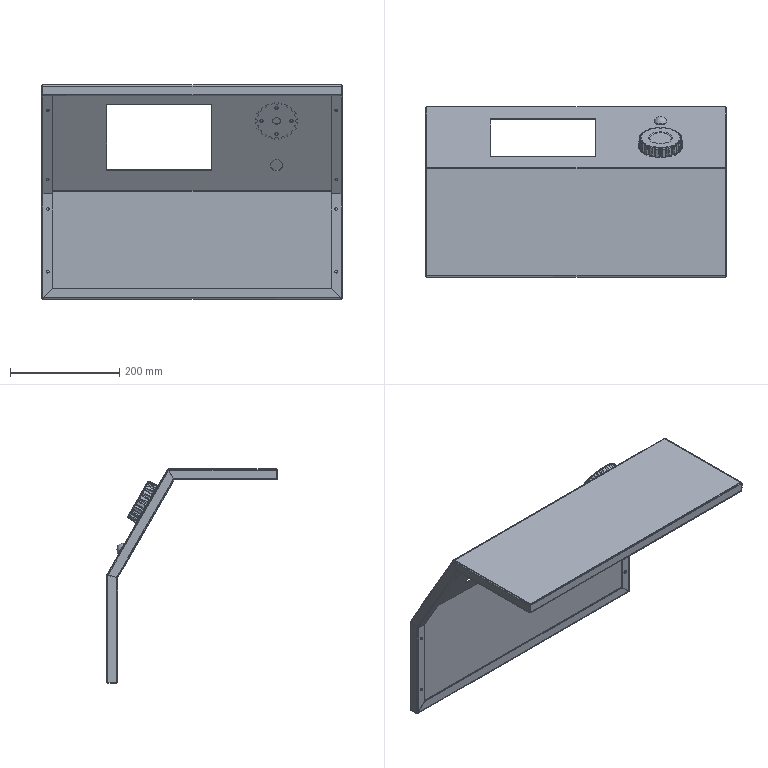Part | SolidWorks | features ICE 9, EdgeFlange 2, Fillet 2, CirPattern 1, Dome 1, FlatPattern 1, Fold 1, SMBaseFlange 1, SheetMetal 1, UnFold 1 | 3 solids | 556 faces | box 549 x 311.751 x 391.2 mm | volume 563037 mm3 | torus 162 | spline 144 | plane 114 | cylinder 74 | cone 60 | sphere 2 | commonest cylinder face diameters 5 x24 2 x18 4.4 x18 6 x8 23 x4 14 x2